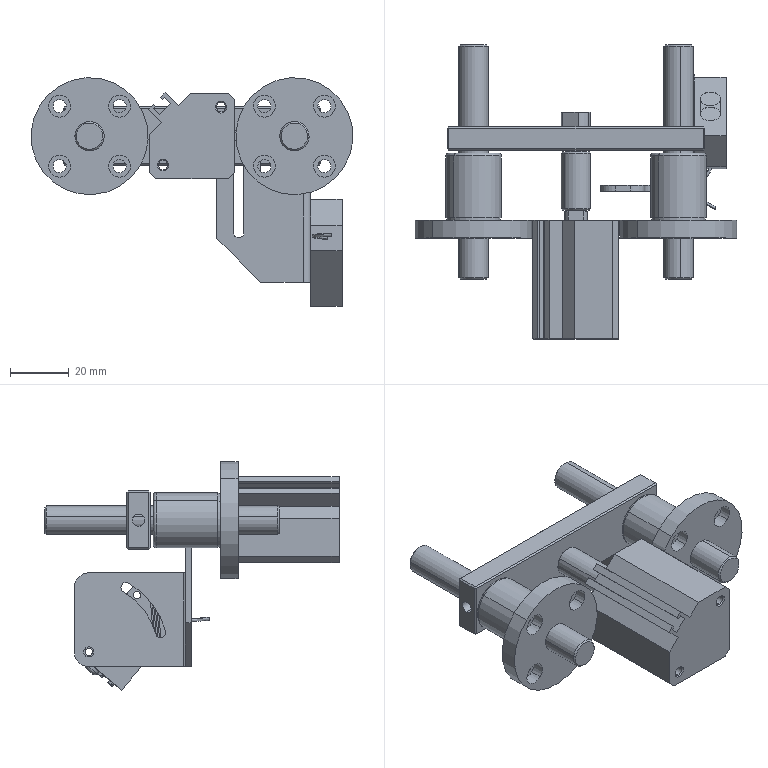Part | SolidWorks | 11 solids | 324 faces | box 110 x 100.5 x 78.14 mm | volume 89945 mm3 | plane 150 | cylinder 126 | cone 40 | torus 6 | spline 2 | commonest cylinder face diameters 10 x22 4.5 x16 7.5 x16 3.5 x10 2 x6 7 x6